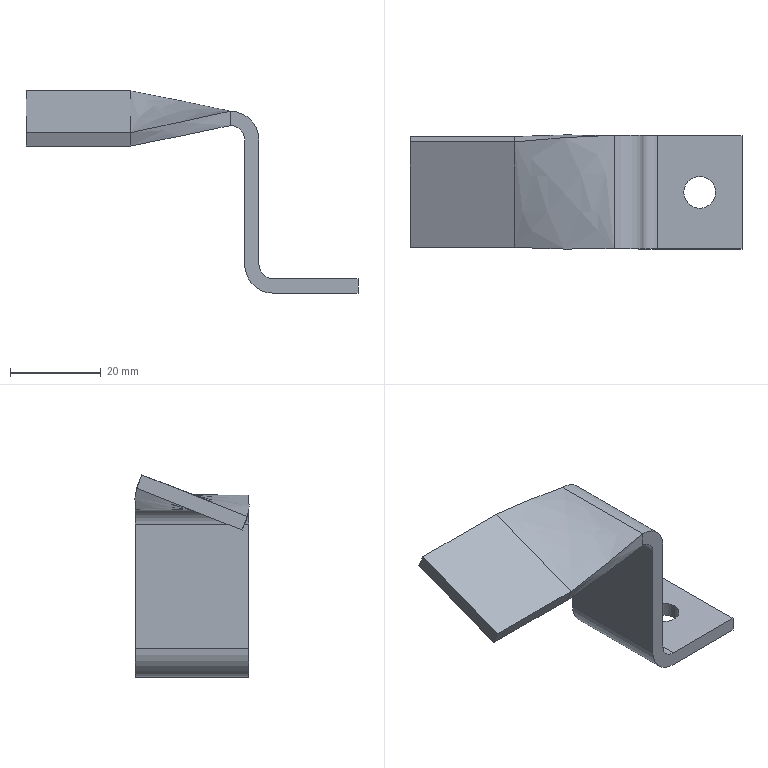Part | SolidWorks | features BaseBody 1 | 1 solid | 24 faces | box 73.18 x 25.199 x 44.598 mm | volume 8281 mm3 | plane 14 | cylinder 6 | spline 4 | commonest cylinder face diameters 6.34 x2 7 x2 12.68 x2
STEP:
#1=CARTESIAN_POINT('',(1.209,1.044,3.17));
#2=VERTEX_POINT('',#1);
#3=CARTESIAN_POINT('',(-5.791,1.044,3.17));
#4=VERTEX_POINT('',#3);
#5=CARTESIAN_POINT('',(-2.291,1.044,3.17));
#6=DIRECTION('',(0.,0.,-1.));
#7=DIRECTION('',(-1.,0.,0.));
#8=AXIS2_PLACEMENT_3D('',#5,#6,#7);
#9=CIRCLE('',#8,3.5);
#10=EDGE_CURVE('',#2,#4,#9,.T.);
#11=ORIENTED_EDGE('',*,*,#10,.F.);
#12=CARTESIAN_POINT('',(1.209,1.044,0.));
#13=VERTEX_POINT('',#12);
#14=CARTESIAN_POINT('',(1.209,1.044,89.394));
#15=DIRECTION('',(0.,0.,-1.));
#16=VECTOR('',#15,1000.);
#17=LINE('',#14,#16);
#18=EDGE_CURVE('',#2,#13,#17,.T.);
#19=ORIENTED_EDGE('',*,*,#18,.T.);
#20=CARTESIAN_POINT('',(-5.791,1.044,0.));
#21=VERTEX_POINT('',#20);
#22=CARTESIAN_POINT('',(-2.291,1.044,0.));
#23=DIRECTION('',(0.,0.,-1.));
#24=DIRECTION('',(-1.,0.,0.));
#25=AXIS2_PLACEMENT_3D('',#22,#23,#24);
#26=CIRCLE('',#25,3.5);
#27=EDGE_CURVE('',#13,#21,#26,.T.);
#28=ORIENTED_EDGE('',*,*,#27,.T.);
#29=CARTESIAN_POINT('',(-5.791,1.044,89.394));
#30=DIRECTION('',(0.,0.,-1.));
#31=VECTOR('',#30,1000.);
#32=LINE('',#29,#31);
#33=EDGE_CURVE('',#4,#21,#32,.T.);
#34=ORIENTED_EDGE('',*,*,#33,.F.);
#35=EDGE_LOOP('',(#11,#19,#28,#34));
#36=FACE_OUTER_BOUND('',#35,.T.);
#37=CARTESIAN_POINT('',(-2.291,1.044,89.394));
#38=DIRECTION('',(0.,0.,-1.));
#39=DIRECTION('',(-1.,0.,0.));
#40=AXIS2_PLACEMENT_3D('',#37,#38,#39);
#41=CYLINDRICAL_SURFACE('',#40,3.5);
#42=ADVANCED_FACE('',(#36),#41,.F.);
#43=CARTESIAN_POINT('',(-14.791,-11.456,6.34));
#44=VERTEX_POINT('',#43);
#45=CARTESIAN_POINT('',(-14.791,13.544,6.34));
#46=VERTEX_POINT('',#45);
#47=CARTESIAN_POINT('',(-14.791,13.544,6.34));
#48=DIRECTION('',(0.,1.,0.));
#49=VECTOR('',#48,1000.);
#50=LINE('',#47,#49);
#51=EDGE_CURVE('',#44,#46,#50,.T.);
#52=ORIENTED_EDGE('',*,*,#51,.T.);
#53=CARTESIAN_POINT('',(-14.791,13.544,33.76));
#54=VERTEX_POINT('',#53);
#55=CARTESIAN_POINT('',(-14.791,13.544,40.1));
#56=DIRECTION('',(0.,0.,1.));
#57=VECTOR('',#56,1000.);
#58=LINE('',#55,#57);
#59=EDGE_CURVE('',#46,#54,#58,.T.);
#60=ORIENTED_EDGE('',*,*,#59,.T.);
#61=CARTESIAN_POINT('',(-14.791,-11.456,33.76));
#62=VERTEX_POINT('',#61);
#63=CARTESIAN_POINT('',(-14.791,13.544,33.76));
#64=DIRECTION('',(0.,-1.,0.));
#65=VECTOR('',#64,1000.);
#66=LINE('',#63,#65);
#67=EDGE_CURVE('',#54,#62,#66,.T.);
#68=ORIENTED_EDGE('',*,*,#67,.T.);
#69=CARTESIAN_POINT('',(-14.791,-11.456,40.1));
#70=DIRECTION('',(0.,0.,-1.));
#71=VECTOR('',#70,1000.);
#72=LINE('',#69,#71);
#73=EDGE_CURVE('',#62,#44,#72,.T.);
#74=ORIENTED_EDGE('',*,*,#73,.T.);
#75=EDGE_LOOP('',(#52,#60,#68,#74));
#76=FACE_OUTER_BOUND('',#75,.T.);
#77=CARTESIAN_POINT('',(-14.791,13.544,40.1));
#78=DIRECTION('',(1.,0.,0.));
#79=DIRECTION('',(0.,1.,0.));
#80=AXIS2_PLACEMENT_3D('',#77,#78,#79);
#81=PLANE('',#80);
#82=ADVANCED_FACE('',(#76),#81,.T.);
#83=CARTESIAN_POINT('',(-17.961,13.544,6.34));
#84=VERTEX_POINT('',#83);
#85=CARTESIAN_POINT('',(-17.961,13.544,33.76));
#86=VERTEX_POINT('',#85);
#87=CARTESIAN_POINT('',(-17.961,13.544,38.515));
#88=DIRECTION('',(0.,0.,1.));
#89=VECTOR('',#88,1000.);
#90=LINE('',#87,#89);
#91=EDGE_CURVE('',#84,#86,#90,.T.);
#92=ORIENTED_EDGE('',*,*,#91,.T.);
#93=CARTESIAN_POINT('',(-21.131,13.544,36.93));
#94=VERTEX_POINT('',#93);
#95=CARTESIAN_POINT('',(-21.131,13.544,33.76));
#96=DIRECTION('',(0.,-1.,0.));
#97=DIRECTION('',(1.,0.,0.));
#98=AXIS2_PLACEMENT_3D('',#95,#96,#97);
#99=CIRCLE('',#98,3.17);
#100=EDGE_CURVE('',#86,#94,#99,.T.);
#101=ORIENTED_EDGE('',*,*,#100,.T.);
#102=CARTESIAN_POINT('',(-21.141,13.544,36.93));
#103=VERTEX_POINT('',#102);
#104=CARTESIAN_POINT('',(-21.141,13.544,36.93));
#105=DIRECTION('',(1.,0.,0.));
#106=VECTOR('',#105,1000.);
#107=LINE('',#104,#106);
#108=EDGE_CURVE('',#103,#94,#107,.T.);
#109=ORIENTED_EDGE('',*,*,#108,.F.);
#110=CARTESIAN_POINT('',(-21.141,13.544,40.1));
#111=VERTEX_POINT('',#110);
#112=CARTESIAN_POINT('',(-21.141,13.544,38.515));
#113=DIRECTION('',(0.,0.,-1.));
#114=VECTOR('',#113,1000.);
#115=LINE('',#112,#114);
#116=EDGE_CURVE('',#111,#103,#115,.T.);
#117=ORIENTED_EDGE('',*,*,#116,.F.);
#118=CARTESIAN_POINT('',(-21.131,13.544,40.1));
#119=VERTEX_POINT('',#118);
#120=CARTESIAN_POINT('',(-14.791,13.544,40.1));
#121=DIRECTION('',(-1.,0.,0.));
#122=VECTOR('',#121,1000.);
#123=LINE('',#120,#122);
#124=EDGE_CURVE('',#119,#111,#123,.T.);
#125=ORIENTED_EDGE('',*,*,#124,.F.);
#126=CARTESIAN_POINT('',(-21.131,13.544,33.76));
#127=DIRECTION('',(0.,1.,0.));
#128=DIRECTION('',(1.,0.,0.));
#129=AXIS2_PLACEMENT_3D('',#126,#127,#128);
#130=CIRCLE('',#129,6.34);
#131=EDGE_CURVE('',#119,#54,#130,.T.);
#132=ORIENTED_EDGE('',*,*,#131,.T.);
#133=ORIENTED_EDGE('',*,*,#59,.F.);
#134=CARTESIAN_POINT('',(-11.621,13.544,3.17));
#135=VERTEX_POINT('',#134);
#136=CARTESIAN_POINT('',(-11.621,13.544,6.34));
#137=DIRECTION('',(0.,-1.,0.));
#138=DIRECTION('',(-1.,0.,0.));
#139=AXIS2_PLACEMENT_3D('',#136,#137,#138);
#140=CIRCLE('',#139,3.17);
#141=EDGE_CURVE('',#46,#135,#140,.T.);
#142=ORIENTED_EDGE('',*,*,#141,.T.);
#143=CARTESIAN_POINT('',(7.039,13.544,3.17));
#144=VERTEX_POINT('',#143);
#145=CARTESIAN_POINT('',(-17.966,13.544,3.17));
#146=DIRECTION('',(1.,0.,0.));
#147=VECTOR('',#146,1000.);
#148=LINE('',#145,#147);
#149=EDGE_CURVE('',#135,#144,#148,.T.);
#150=ORIENTED_EDGE('',*,*,#149,.T.);
#151=CARTESIAN_POINT('',(7.039,13.544,0.));
#152=VERTEX_POINT('',#151);
#153=CARTESIAN_POINT('',(7.039,13.544,38.515));
#154=DIRECTION('',(0.,0.,-1.));
#155=VECTOR('',#154,1000.);
#156=LINE('',#153,#155);
#157=EDGE_CURVE('',#144,#152,#156,.T.);
#158=ORIENTED_EDGE('',*,*,#157,.T.);
#159=CARTESIAN_POINT('',(-11.621,13.544,0.));
#160=VERTEX_POINT('',#159);
#161=CARTESIAN_POINT('',(-17.966,13.544,0.));
#162=DIRECTION('',(-1.,0.,0.));
#163=VECTOR('',#162,1000.);
#164=LINE('',#161,#163);
#165=EDGE_CURVE('',#152,#160,#164,.T.);
#166=ORIENTED_EDGE('',*,*,#165,.T.);
#167=CARTESIAN_POINT('',(-11.621,13.544,6.34));
#168=DIRECTION('',(0.,1.,0.));
#169=DIRECTION('',(-1.,0.,0.));
#170=AXIS2_PLACEMENT_3D('',#167,#168,#169);
#171=CIRCLE('',#170,6.34);
#172=EDGE_CURVE('',#160,#84,#171,.T.);
#173=ORIENTED_EDGE('',*,*,#172,.T.);
#174=EDGE_LOOP('',(#92,#101,#109,#117,#125,#132,#133,#142,#150,#158,#166,#173));
#175=FACE_OUTER_BOUND('',#174,.T.);
#176=CARTESIAN_POINT('',(-17.966,13.544,38.515));
#177=DIRECTION('',(0.,1.,0.));
#178=DIRECTION('',(0.,0.,1.));
#179=AXIS2_PLACEMENT_3D('',#176,#177,#178);
#180=PLANE('',#179);
#181=ADVANCED_FACE('',(#175),#180,.T.);
#182=CARTESIAN_POINT('',(-11.621,-11.456,3.17));
#183=VERTEX_POINT('',#182);
#184=CARTESIAN_POINT('',(-11.621,-11.456,6.34));
#185=DIRECTION('',(0.,1.,0.));
#186=DIRECTION('',(-1.,0.,0.));
#187=AXIS2_PLACEMENT_3D('',#184,#185,#186);
#188=CIRCLE('',#187,3.17);
#189=EDGE_CURVE('',#183,#44,#188,.T.);
#190=ORIENTED_EDGE('',*,*,#189,.F.);
#191=CARTESIAN_POINT('',(-11.621,1.044,3.17));
#192=DIRECTION('',(0.,-1.,0.));
#193=VECTOR('',#192,1000.);
#194=LINE('',#191,#193);
#195=EDGE_CURVE('',#135,#183,#194,.T.);
#196=ORIENTED_EDGE('',*,*,#195,.F.);
#197=ORIENTED_EDGE('',*,*,#141,.F.);
#198=ORIENTED_EDGE('',*,*,#51,.F.);
#199=EDGE_LOOP('',(#190,#196,#197,#198));
#200=FACE_OUTER_BOUND('',#199,.T.);
#201=CARTESIAN_POINT('',(-11.621,1.044,6.34));
#202=DIRECTION('',(0.,1.,0.));
#203=DIRECTION('',(-1.,0.,0.));
#204=AXIS2_PLACEMENT_3D('',#201,#202,#203);
#205=CYLINDRICAL_SURFACE('',#204,3.17);
#206=ADVANCED_FACE('',(#200),#205,.F.);
#207=CARTESIAN_POINT('',(-21.141,-11.456,36.93));
#208=VERTEX_POINT('',#207);
#209=CARTESIAN_POINT('',(-21.141,-11.456,40.1));
#210=VERTEX_POINT('',#209);
#211=CARTESIAN_POINT('',(-21.141,-11.456,38.515));
#212=DIRECTION('',(0.,0.,1.));
#213=VECTOR('',#212,1000.);
#214=LINE('',#211,#213);
#215=EDGE_CURVE('',#208,#210,#214,.T.);
#216=ORIENTED_EDGE('',*,*,#215,.F.);
#217=CARTESIAN_POINT('',(-21.131,-11.456,36.93));
#218=VERTEX_POINT('',#217);
#219=CARTESIAN_POINT('',(-21.141,-11.456,36.93));
#220=DIRECTION('',(-1.,0.,0.));
#221=VECTOR('',#220,1000.);
#222=LINE('',#219,#221);
#223=EDGE_CURVE('',#218,#208,#222,.T.);
#224=ORIENTED_EDGE('',*,*,#223,.F.);
#225=CARTESIAN_POINT('',(-17.961,-11.456,33.76));
#226=VERTEX_POINT('',#225);
#227=CARTESIAN_POINT('',(-21.131,-11.456,33.76));
#228=DIRECTION('',(0.,-1.,0.));
#229=DIRECTION('',(1.,0.,0.));
#230=AXIS2_PLACEMENT_3D('',#227,#228,#229);
#231=CIRCLE('',#230,3.17);
#232=EDGE_CURVE('',#226,#218,#231,.T.);
#233=ORIENTED_EDGE('',*,*,#232,.F.);
#234=CARTESIAN_POINT('',(-17.961,-11.456,6.34));
#235=VERTEX_POINT('',#234);
#236=CARTESIAN_POINT('',(-17.961,-11.456,38.515));
#237=DIRECTION('',(0.,0.,1.));
#238=VECTOR('',#237,1000.);
#239=LINE('',#236,#238);
#240=EDGE_CURVE('',#235,#226,#239,.T.);
#241=ORIENTED_EDGE('',*,*,#240,.F.);
#242=CARTESIAN_POINT('',(-11.621,-11.456,0.));
#243=VERTEX_POINT('',#242);
#244=CARTESIAN_POINT('',(-11.621,-11.456,6.34));
#245=DIRECTION('',(0.,1.,0.));
#246=DIRECTION('',(-1.,0.,0.));
#247=AXIS2_PLACEMENT_3D('',#244,#245,#246);
#248=CIRCLE('',#247,6.34);
#249=EDGE_CURVE('',#243,#235,#248,.T.);
#250=ORIENTED_EDGE('',*,*,#249,.F.);
#251=CARTESIAN_POINT('',(7.039,-11.456,0.));
#252=VERTEX_POINT('',#251);
#253=CARTESIAN_POINT('',(-17.966,-11.456,0.));
#254=DIRECTION('',(-1.,0.,0.));
#255=VECTOR('',#254,1000.);
#256=LINE('',#253,#255);
#257=EDGE_CURVE('',#252,#243,#256,.T.);
#258=ORIENTED_EDGE('',*,*,#257,.F.);
#259=CARTESIAN_POINT('',(7.039,-11.456,3.17));
#260=VERTEX_POINT('',#259);
#261=CARTESIAN_POINT('',(7.039,-11.456,38.515));
#262=DIRECTION('',(0.,0.,-1.));
#263=VECTOR('',#262,1000.);
#264=LINE('',#261,#263);
#265=EDGE_CURVE('',#260,#252,#264,.T.);
#266=ORIENTED_EDGE('',*,*,#265,.F.);
#267=CARTESIAN_POINT('',(-17.966,-11.456,3.17));
#268=DIRECTION('',(1.,0.,0.));
#269=VECTOR('',#268,1000.);
#270=LINE('',#267,#269);
#271=EDGE_CURVE('',#183,#260,#270,.T.);
#272=ORIENTED_EDGE('',*,*,#271,.F.);
#273=ORIENTED_EDGE('',*,*,#189,.T.);
#274=ORIENTED_EDGE('',*,*,#73,.F.);
#275=CARTESIAN_POINT('',(-21.131,-11.456,40.1));
#276=VERTEX_POINT('',#275);
#277=CARTESIAN_POINT('',(-21.131,-11.456,33.76));
#278=DIRECTION('',(0.,1.,0.));
#279=DIRECTION('',(1.,0.,0.));
#280=AXIS2_PLACEMENT_3D('',#277,#278,#279);
#281=CIRCLE('',#280,6.34);
#282=EDGE_CURVE('',#276,#62,#281,.T.);
#283=ORIENTED_EDGE('',*,*,#282,.F.);
#284=CARTESIAN_POINT('',(-14.791,-11.456,40.1));
#285=DIRECTION('',(1.,0.,0.));
#286=VECTOR('',#285,1000.);
#287=LINE('',#284,#286);
#288=EDGE_CURVE('',#210,#276,#287,.T.);
#289=ORIENTED_EDGE('',*,*,#288,.F.);
#290=EDGE_LOOP('',(#216,#224,#233,#241,#250,#258,#266,#272,#273,#274,#283,#289));
#291=FACE_OUTER_BOUND('',#290,.T.);
#292=CARTESIAN_POINT('',(-17.966,-11.456,38.515));
#293=DIRECTION('',(0.,1.,0.));
#294=DIRECTION('',(0.,0.,1.));
#295=AXIS2_PLACEMENT_3D('',#292,#293,#294);
#296=PLANE('',#295);
#297=ADVANCED_FACE('',(#291),#296,.F.);
#298=ORIENTED_EDGE('',*,*,#67,.F.);
#299=ORIENTED_EDGE('',*,*,#131,.F.);
#300=CARTESIAN_POINT('',(-21.131,1.044,40.1));
#301=DIRECTION('',(0.,-1.,0.));
#302=VECTOR('',#301,1000.);
#303=LINE('',#300,#302);
#304=EDGE_CURVE('',#119,#276,#303,.T.);
#305=ORIENTED_EDGE('',*,*,#304,.T.);
#306=ORIENTED_EDGE('',*,*,#282,.T.);
#307=EDGE_LOOP('',(#298,#299,#305,#306));
#308=FACE_OUTER_BOUND('',#307,.T.);
#309=CARTESIAN_POINT('',(-21.131,1.044,33.76));
#310=DIRECTION('',(0.,-1.,0.));
#311=DIRECTION('',(1.,0.,0.));
#312=AXIS2_PLACEMENT_3D('',#309,#310,#311);
#313=CYLINDRICAL_SURFACE('',#312,6.34);
#314=ADVANCED_FACE('',(#308),#313,.T.);
#315=ORIENTED_EDGE('',*,*,#100,.F.);
#316=CARTESIAN_POINT('',(-17.961,1.044,33.76));
#317=DIRECTION('',(0.,1.,0.));
#318=VECTOR('',#317,1000.);
#319=LINE('',#316,#318);
#320=EDGE_CURVE('',#226,#86,#319,.T.);
#321=ORIENTED_EDGE('',*,*,#320,.F.);
#322=ORIENTED_EDGE('',*,*,#232,.T.);
#323=CARTESIAN_POINT('',(-21.131,1.044,36.93));
#324=DIRECTION('',(0.,-1.,0.));
#325=VECTOR('',#324,1000.);
#326=LINE('',#323,#325);
#327=EDGE_CURVE('',#94,#218,#326,.T.);
#328=ORIENTED_EDGE('',*,*,#327,.F.);
#329=EDGE_LOOP('',(#315,#321,#322,#328));
#330=FACE_OUTER_BOUND('',#329,.T.);
#331=CARTESIAN_POINT('',(-21.131,1.044,33.76));
#332=DIRECTION('',(0.,-1.,0.));
#333=DIRECTION('',(1.,0.,0.));
#334=AXIS2_PLACEMENT_3D('',#331,#332,#333);
#335=CYLINDRICAL_SURFACE('',#334,3.17);
#336=ADVANCED_FACE('',(#330),#335,.F.);
#337=CARTESIAN_POINT('',(-17.961,13.544,6.34));
#338=DIRECTION('',(0.,-1.,0.));
#339=VECTOR('',#338,1000.);
#340=LINE('',#337,#339);
#341=EDGE_CURVE('',#84,#235,#340,.T.);
#342=ORIENTED_EDGE('',*,*,#341,.T.);
#343=ORIENTED_EDGE('',*,*,#240,.T.);
#344=ORIENTED_EDGE('',*,*,#320,.T.);
#345=ORIENTED_EDGE('',*,*,#91,.F.);
#346=EDGE_LOOP('',(#342,#343,#344,#345));
#347=FACE_OUTER_BOUND('',#346,.T.);
#348=CARTESIAN_POINT('',(-17.961,13.544,0.));
#349=DIRECTION('',(-1.,0.,0.));
#350=DIRECTION('',(0.,-1.,0.));
#351=AXIS2_PLACEMENT_3D('',#348,#349,#350);
#352=PLANE('',#351);
#353=ADVANCED_FACE('',(#347),#352,.T.);
#354=CARTESIAN_POINT('',(-11.621,1.044,0.));
#355=DIRECTION('',(0.,-1.,0.));
#356=VECTOR('',#355,1000.);
#357=LINE('',#354,#356);
#358=EDGE_CURVE('',#160,#243,#357,.T.);
#359=ORIENTED_EDGE('',*,*,#358,.T.);
#360=ORIENTED_EDGE('',*,*,#249,.T.);
#361=ORIENTED_EDGE('',*,*,#341,.F.);
#362=ORIENTED_EDGE('',*,*,#172,.F.);
#363=EDGE_LOOP('',(#359,#360,#361,#362));
#364=FACE_OUTER_BOUND('',#363,.T.);
#365=CARTESIAN_POINT('',(-11.621,1.044,6.34));
#366=DIRECTION('',(0.,1.,0.));
#367=DIRECTION('',(-1.,0.,0.));
#368=AXIS2_PLACEMENT_3D('',#365,#366,#367);
#369=CYLINDRICAL_SURFACE('',#368,6.34);
#370=ADVANCED_FACE('',(#364),#369,.T.);
#371=CARTESIAN_POINT('',(-2.291,1.044,0.));
#372=DIRECTION('',(0.,0.,-1.));
#373=DIRECTION('',(-1.,0.,0.));
#374=AXIS2_PLACEMENT_3D('',#371,#372,#373);
#375=CIRCLE('',#374,3.5);
#376=EDGE_CURVE('',#21,#13,#375,.T.);
#377=ORIENTED_EDGE('',*,*,#376,.F.);
#378=ORIENTED_EDGE('',*,*,#27,.F.);
#379=EDGE_LOOP('',(#377,#378));
#380=FACE_BOUND('',#379,.T.);
#381=ORIENTED_EDGE('',*,*,#165,.F.);
#382=CARTESIAN_POINT('',(7.039,1.044,0.));
#383=DIRECTION('',(0.,1.,0.));
#384=VECTOR('',#383,1000.);
#385=LINE('',#382,#384);
#386=EDGE_CURVE('',#252,#152,#385,.T.);
#387=ORIENTED_EDGE('',*,*,#386,.F.);
#388=ORIENTED_EDGE('',*,*,#257,.T.);
#389=ORIENTED_EDGE('',*,*,#358,.F.);
#390=EDGE_LOOP('',(#381,#387,#388,#389));
#391=FACE_OUTER_BOUND('',#390,.T.);
#392=CARTESIAN_POINT('',(-5.461,1.044,0.));
#393=DIRECTION('',(0.,0.,1.));
#394=DIRECTION('',(1.,0.,0.));
#395=AXIS2_PLACEMENT_3D('',#392,#393,#394);
#396=PLANE('',#395);
#397=ADVANCED_FACE('',(#380,#391),#396,.F.);
#398=ORIENTED_EDGE('',*,*,#386,.T.);
#399=ORIENTED_EDGE('',*,*,#157,.F.);
#400=CARTESIAN_POINT('',(7.039,13.544,3.17));
#401=DIRECTION('',(0.,-1.,0.));
#402=VECTOR('',#401,1000.);
#403=LINE('',#400,#402);
#404=EDGE_CURVE('',#144,#260,#403,.T.);
#405=ORIENTED_EDGE('',*,*,#404,.T.);
#406=ORIENTED_EDGE('',*,*,#265,.T.);
#407=EDGE_LOOP('',(#398,#399,#405,#406));
#408=FACE_OUTER_BOUND('',#407,.T.);
#409=CARTESIAN_POINT('',(7.039,13.544,0.));
#410=DIRECTION('',(1.,0.,0.));
#411=DIRECTION('',(0.,0.,-1.));
#412=AXIS2_PLACEMENT_3D('',#409,#410,#411);
#413=PLANE('',#412);
#414=ADVANCED_FACE('',(#408),#413,.T.);
#415=CARTESIAN_POINT('',(-2.291,1.044,3.17));
#416=DIRECTION('',(0.,0.,-1.));
#417=DIRECTION('',(-1.,0.,0.));
#418=AXIS2_PLACEMENT_3D('',#415,#416,#417);
#419=CIRCLE('',#418,3.5);
#420=EDGE_CURVE('',#4,#2,#419,.T.);
#421=ORIENTED_EDGE('',*,*,#420,.T.);
#422=ORIENTED_EDGE('',*,*,#10,.T.);
#423=EDGE_LOOP('',(#421,#422));
#424=FACE_BOUND('',#423,.T.);
#425=ORIENTED_EDGE('',*,*,#404,.F.);
#426=ORIENTED_EDGE('',*,*,#149,.F.);
#427=ORIENTED_EDGE('',*,*,#195,.T.);
#428=ORIENTED_EDGE('',*,*,#271,.T.);
#429=EDGE_LOOP('',(#425,#426,#427,#428));
#430=FACE_OUTER_BOUND('',#429,.T.);
#431=CARTESIAN_POINT('',(-5.461,1.044,3.17));
#432=DIRECTION('',(0.,0.,1.));
#433=DIRECTION('',(1.,0.,0.));
#434=AXIS2_PLACEMENT_3D('',#431,#432,#433);
#435=PLANE('',#434);
#436=ADVANCED_FACE('',(#424,#430),#435,.T.);
#437=CARTESIAN_POINT('',(-21.141,-11.456,40.1));
#438=DIRECTION('',(0.,-1.,0.));
#439=VECTOR('',#438,1000.);
#440=LINE('',#437,#439);
#441=EDGE_CURVE('',#111,#210,#440,.T.);
#442=ORIENTED_EDGE('',*,*,#441,.T.);
#443=ORIENTED_EDGE('',*,*,#288,.T.);
#444=ORIENTED_EDGE('',*,*,#304,.F.);
#445=ORIENTED_EDGE('',*,*,#124,.T.);
#446=EDGE_LOOP('',(#442,#443,#444,#445));
#447=FACE_OUTER_BOUND('',#446,.T.);
#448=CARTESIAN_POINT('',(-14.791,-11.456,40.1));
#449=DIRECTION('',(0.,0.,1.));
#450=DIRECTION('',(1.,0.,0.));
#451=AXIS2_PLACEMENT_3D('',#448,#449,#450);
#452=PLANE('',#451);
#453=ADVANCED_FACE('',(#447),#452,.T.);
#454=CARTESIAN_POINT('',(-21.141,-11.456,36.93));
#455=DIRECTION('',(0.,1.,0.));
#456=VECTOR('',#455,1000.);
#457=LINE('',#454,#456);
#458=EDGE_CURVE('',#208,#103,#457,.T.);
#459=ORIENTED_EDGE('',*,*,#458,.T.);
#460=ORIENTED_EDGE('',*,*,#108,.T.);
#461=ORIENTED_EDGE('',*,*,#327,.T.);
#462=ORIENTED_EDGE('',*,*,#223,.T.);
#463=EDGE_LOOP('',(#459,#460,#461,#462));
#464=FACE_OUTER_BOUND('',#463,.T.);
#465=CARTESIAN_POINT('',(-21.141,-11.456,36.93));
#466=DIRECTION('',(0.,0.,-1.));
#467=DIRECTION('',(-1.,0.,0.));
#468=AXIS2_PLACEMENT_3D('',#465,#466,#467);
#469=PLANE('',#468);
#470=ADVANCED_FACE('',(#464),#469,.T.);
#471=ORIENTED_EDGE('',*,*,#18,.F.);
#472=ORIENTED_EDGE('',*,*,#420,.F.);
#473=ORIENTED_EDGE('',*,*,#33,.T.);
#474=ORIENTED_EDGE('',*,*,#376,.T.);
#475=EDGE_LOOP('',(#471,#472,#473,#474));
#476=FACE_OUTER_BOUND('',#475,.T.);
#477=CARTESIAN_POINT('',(-2.291,1.044,89.394));
#478=DIRECTION('',(0.,0.,-1.));
#479=DIRECTION('',(-1.,0.,0.));
#480=AXIS2_PLACEMENT_3D('',#477,#478,#479);
#481=CYLINDRICAL_SURFACE('',#480,3.5);
#482=ADVANCED_FACE('',(#476),#481,.F.);
#483=ORIENTED_EDGE('',*,*,#441,.F.);
#484=CARTESIAN_POINT('',(-43.141,12.078,44.598));
#485=VERTEX_POINT('',#484);
#486=CARTESIAN_POINT('',(-21.141,13.544,40.1));
#487=CARTESIAN_POINT('',(-28.474,13.344,41.674));
#488=CARTESIAN_POINT('',(-35.808,12.844,43.209));
#489=CARTESIAN_POINT('',(-43.141,12.078,44.598));
#490=B_SPLINE_CURVE_WITH_KNOTS('',3,(#486,#487,#488,#489),.UNSPECIFIED.,.F.,.F.,(4,4),(0.,0.3777),.UNSPECIFIED.);
#491=EDGE_CURVE('',#111,#485,#490,.T.);
#492=ORIENTED_EDGE('',*,*,#491,.T.);
#493=CARTESIAN_POINT('',(-43.141,-11.16,35.379));
#494=VERTEX_POINT('',#493);
#495=CARTESIAN_POINT('',(-43.141,0.4592,39.988));
#496=DIRECTION('',(0.,-0.9295,-0.3688));
#497=VECTOR('',#496,1000.);
#498=LINE('',#495,#497);
#499=EDGE_CURVE('',#485,#494,#498,.T.);
#500=ORIENTED_EDGE('',*,*,#499,.T.);
#501=CARTESIAN_POINT('',(-43.141,-11.16,35.379));
#502=CARTESIAN_POINT('',(-35.808,-11.555,36.915));
#503=CARTESIAN_POINT('',(-28.474,-11.656,38.526));
#504=CARTESIAN_POINT('',(-21.141,-11.456,40.1));
#505=B_SPLINE_CURVE_WITH_KNOTS('',3,(#501,#502,#503,#504),.UNSPECIFIED.,.F.,.F.,(4,4),(0.,0.3777),.UNSPECIFIED.);
#506=EDGE_CURVE('',#494,#210,#505,.T.);
#507=ORIENTED_EDGE('',*,*,#506,.T.);
#508=EDGE_LOOP('',(#483,#492,#500,#507));
#509=FACE_OUTER_BOUND('',#508,.T.);
#510=CARTESIAN_POINT('',(-21.141,-11.456,40.1));
#511=CARTESIAN_POINT('',(-28.474,-11.656,38.526));
#512=CARTESIAN_POINT('',(-35.808,-11.555,36.915));
#513=CARTESIAN_POINT('',(-43.141,-11.16,35.379));
#514=CARTESIAN_POINT('',(-21.141,-3.123,40.1));
#515=CARTESIAN_POINT('',(-28.474,-3.323,39.575));
#516=CARTESIAN_POINT('',(-35.808,-3.422,39.013));
#517=CARTESIAN_POINT('',(-43.141,-3.414,38.452));
#518=CARTESIAN_POINT('',(-21.141,5.21,40.1));
#519=CARTESIAN_POINT('',(-28.474,5.011,40.625));
#520=CARTESIAN_POINT('',(-35.808,4.711,41.111));
#521=CARTESIAN_POINT('',(-43.141,4.332,41.525));
#522=CARTESIAN_POINT('',(-21.141,13.544,40.1));
#523=CARTESIAN_POINT('',(-28.474,13.344,41.674));
#524=CARTESIAN_POINT('',(-35.808,12.844,43.209));
#525=CARTESIAN_POINT('',(-43.141,12.078,44.598));
#526=B_SPLINE_SURFACE_WITH_KNOTS('',3,3,((#510,#511,#512,#513),(#514,#515,#516,#517),(#518,#519,#520,#521),(#522,#523,#524,#525)),.UNSPECIFIED.,.F.,.F.,.F.,(4,4),(4,4),(0.,2.5),(0.,0.3777),.UNSPECIFIED.);
#527=ADVANCED_FACE('',(#509),#526,.T.);
#528=ORIENTED_EDGE('',*,*,#458,.F.);
#529=CARTESIAN_POINT('',(-43.141,-9.991,32.432));
#530=VERTEX_POINT('',#529);
#531=CARTESIAN_POINT('',(-21.141,-11.456,36.93));
#532=CARTESIAN_POINT('',(-28.474,-11.257,35.356));
#533=CARTESIAN_POINT('',(-35.808,-10.757,33.821));
#534=CARTESIAN_POINT('',(-43.141,-9.991,32.432));
#535=B_SPLINE_CURVE_WITH_KNOTS('',3,(#531,#532,#533,#534),.UNSPECIFIED.,.F.,.F.,(4,4),(0.,0.3777),.UNSPECIFIED.);
#536=EDGE_CURVE('',#208,#530,#535,.T.);
#537=ORIENTED_EDGE('',*,*,#536,.T.);
#538=CARTESIAN_POINT('',(-43.141,13.247,41.651));
#539=VERTEX_POINT('',#538);
#540=CARTESIAN_POINT('',(-43.141,1.628,37.042));
#541=DIRECTION('',(0.,0.9295,0.3688));
#542=VECTOR('',#541,1000.);
#543=LINE('',#540,#542);
#544=EDGE_CURVE('',#530,#539,#543,.T.);
#545=ORIENTED_EDGE('',*,*,#544,.T.);
#546=CARTESIAN_POINT('',(-43.141,13.247,41.651));
#547=CARTESIAN_POINT('',(-35.808,13.642,40.115));
#548=CARTESIAN_POINT('',(-28.474,13.743,38.504));
#549=CARTESIAN_POINT('',(-21.141,13.544,36.93));
#550=B_SPLINE_CURVE_WITH_KNOTS('',3,(#546,#547,#548,#549),.UNSPECIFIED.,.F.,.F.,(4,4),(0.,0.3777),.UNSPECIFIED.);
#551=EDGE_CURVE('',#539,#103,#550,.T.);
#552=ORIENTED_EDGE('',*,*,#551,.T.);
#553=EDGE_LOOP('',(#528,#537,#545,#552));
#554=FACE_OUTER_BOUND('',#553,.T.);
#555=CARTESIAN_POINT('',(-21.141,13.544,36.93));
#556=CARTESIAN_POINT('',(-28.474,13.743,38.504));
#557=CARTESIAN_POINT('',(-35.808,13.642,40.115));
#558=CARTESIAN_POINT('',(-43.141,13.247,41.651));
#559=CARTESIAN_POINT('',(-21.141,5.21,36.93));
#560=CARTESIAN_POINT('',(-28.474,5.41,37.455));
#561=CARTESIAN_POINT('',(-35.808,5.509,38.017));
#562=CARTESIAN_POINT('',(-43.141,5.501,38.578));
#563=CARTESIAN_POINT('',(-21.141,-3.123,36.93));
#564=CARTESIAN_POINT('',(-28.474,-2.923,36.405));
#565=CARTESIAN_POINT('',(-35.808,-2.624,35.919));
#566=CARTESIAN_POINT('',(-43.141,-2.245,35.505));
#567=CARTESIAN_POINT('',(-21.141,-11.456,36.93));
#568=CARTESIAN_POINT('',(-28.474,-11.257,35.356));
#569=CARTESIAN_POINT('',(-35.808,-10.757,33.821));
#570=CARTESIAN_POINT('',(-43.141,-9.991,32.432));
#571=B_SPLINE_SURFACE_WITH_KNOTS('',3,3,((#555,#556,#557,#558),(#559,#560,#561,#562),(#563,#564,#565,#566),(#567,#568,#569,#570)),.UNSPECIFIED.,.F.,.F.,.F.,(4,4),(4,4),(0.,2.5),(0.,0.3777),.UNSPECIFIED.);
#572=ADVANCED_FACE('',(#554),#571,.T.);
#573=ORIENTED_EDGE('',*,*,#116,.T.);
#574=ORIENTED_EDGE('',*,*,#551,.F.);
#575=CARTESIAN_POINT('',(-43.141,13.247,41.651));
#576=DIRECTION('',(0.,0.3688,-0.9295));
#577=VECTOR('',#576,1000.);
#578=LINE('',#575,#577);
#579=EDGE_CURVE('',#485,#539,#578,.T.);
#580=ORIENTED_EDGE('',*,*,#579,.F.);
#581=ORIENTED_EDGE('',*,*,#491,.F.);
#582=EDGE_LOOP('',(#573,#574,#580,#581));
#583=FACE_OUTER_BOUND('',#582,.T.);
#584=CARTESIAN_POINT('',(-21.141,13.544,40.1));
#585=CARTESIAN_POINT('',(-28.474,13.344,41.674));
#586=CARTESIAN_POINT('',(-35.808,12.844,43.209));
#587=CARTESIAN_POINT('',(-43.141,12.078,44.598));
#588=CARTESIAN_POINT('',(-21.141,13.544,39.043));
#589=CARTESIAN_POINT('',(-28.474,13.477,40.617));
#590=CARTESIAN_POINT('',(-35.808,13.11,42.177));
#591=CARTESIAN_POINT('',(-43.141,12.468,43.616));
#592=CARTESIAN_POINT('',(-21.141,13.544,37.987));
#593=CARTESIAN_POINT('',(-28.474,13.61,39.56));
#594=CARTESIAN_POINT('',(-35.808,13.376,41.146));
#595=CARTESIAN_POINT('',(-43.141,12.858,42.633));
#596=CARTESIAN_POINT('',(-21.141,13.544,36.93));
#597=CARTESIAN_POINT('',(-28.474,13.743,38.504));
#598=CARTESIAN_POINT('',(-35.808,13.642,40.115));
#599=CARTESIAN_POINT('',(-43.141,13.247,41.651));
#600=B_SPLINE_SURFACE_WITH_KNOTS('',3,3,((#584,#585,#586,#587),(#588,#589,#590,#591),(#592,#593,#594,#595),(#596,#597,#598,#599)),.UNSPECIFIED.,.F.,.F.,.F.,(4,4),(4,4),(0.,0.317),(0.,0.3777),.UNSPECIFIED.);
#601=ADVANCED_FACE('',(#583),#600,.T.);
#602=ORIENTED_EDGE('',*,*,#215,.T.);
#603=ORIENTED_EDGE('',*,*,#506,.F.);
#604=CARTESIAN_POINT('',(-43.141,-11.16,35.379));
#605=DIRECTION('',(0.,-0.3688,0.9295));
#606=VECTOR('',#605,1000.);
#607=LINE('',#604,#606);
#608=EDGE_CURVE('',#530,#494,#607,.T.);
#609=ORIENTED_EDGE('',*,*,#608,.F.);
#610=ORIENTED_EDGE('',*,*,#536,.F.);
#611=EDGE_LOOP('',(#602,#603,#609,#610));
#612=FACE_OUTER_BOUND('',#611,.T.);
#613=CARTESIAN_POINT('',(-21.141,-11.456,36.93));
#614=CARTESIAN_POINT('',(-28.474,-11.257,35.356));
#615=CARTESIAN_POINT('',(-35.808,-10.757,33.821));
#616=CARTESIAN_POINT('',(-43.141,-9.991,32.432));
#617=CARTESIAN_POINT('',(-21.141,-11.456,37.987));
#618=CARTESIAN_POINT('',(-28.474,-11.39,36.413));
#619=CARTESIAN_POINT('',(-35.808,-11.023,34.853));
#620=CARTESIAN_POINT('',(-43.141,-10.381,33.414));
#621=CARTESIAN_POINT('',(-21.141,-11.456,39.043));
#622=CARTESIAN_POINT('',(-28.474,-11.523,37.47));
#623=CARTESIAN_POINT('',(-35.808,-11.289,35.884));
#624=CARTESIAN_POINT('',(-43.141,-10.77,34.397));
#625=CARTESIAN_POINT('',(-21.141,-11.456,40.1));
#626=CARTESIAN_POINT('',(-28.474,-11.656,38.526));
#627=CARTESIAN_POINT('',(-35.808,-11.555,36.915));
#628=CARTESIAN_POINT('',(-43.141,-11.16,35.379));
#629=B_SPLINE_SURFACE_WITH_KNOTS('',3,3,((#613,#614,#615,#616),(#617,#618,#619,#620),(#621,#622,#623,#624),(#625,#626,#627,#628)),.UNSPECIFIED.,.F.,.F.,.F.,(4,4),(4,4),(0.,0.317),(0.,0.3777),.UNSPECIFIED.);
#630=ADVANCED_FACE('',(#612),#629,.T.);
#631=ORIENTED_EDGE('',*,*,#499,.F.);
#632=CARTESIAN_POINT('',(-66.141,12.078,44.598));
#633=VERTEX_POINT('',#632);
#634=CARTESIAN_POINT('',(-43.141,12.078,44.598));
#635=DIRECTION('',(-1.,0.,0.));
#636=VECTOR('',#635,1000.);
#637=LINE('',#634,#636);
#638=EDGE_CURVE('',#485,#633,#637,.T.);
#639=ORIENTED_EDGE('',*,*,#638,.T.);
#640=CARTESIAN_POINT('',(-66.141,-11.16,35.379));
#641=VERTEX_POINT('',#640);
#642=CARTESIAN_POINT('',(-66.141,12.078,44.598));
#643=DIRECTION('',(0.,-0.9295,-0.3688));
#644=VECTOR('',#643,1000.);
#645=LINE('',#642,#644);
#646=EDGE_CURVE('',#633,#641,#645,.T.);
#647=ORIENTED_EDGE('',*,*,#646,.T.);
#648=CARTESIAN_POINT('',(-43.141,-11.16,35.379));
#649=DIRECTION('',(1.,0.,0.));
#650=VECTOR('',#649,1000.);
#651=LINE('',#648,#650);
#652=EDGE_CURVE('',#641,#494,#651,.T.);
#653=ORIENTED_EDGE('',*,*,#652,.T.);
#654=EDGE_LOOP('',(#631,#639,#647,#653));
#655=FACE_OUTER_BOUND('',#654,.T.);
#656=CARTESIAN_POINT('',(-43.141,12.078,44.598));
#657=DIRECTION('',(0.,-0.3688,0.9295));
#658=DIRECTION('',(0.,-0.9295,-0.3688));
#659=AXIS2_PLACEMENT_3D('',#656,#657,#658);
#660=PLANE('',#659);
#661=ADVANCED_FACE('',(#655),#660,.T.);
#662=ORIENTED_EDGE('',*,*,#544,.F.);
#663=CARTESIAN_POINT('',(-66.141,-9.991,32.432));
#664=VERTEX_POINT('',#663);
#665=CARTESIAN_POINT('',(-43.141,-9.991,32.432));
#666=DIRECTION('',(-1.,0.,0.));
#667=VECTOR('',#666,1000.);
#668=LINE('',#665,#667);
#669=EDGE_CURVE('',#530,#664,#668,.T.);
#670=ORIENTED_EDGE('',*,*,#669,.T.);
#671=CARTESIAN_POINT('',(-66.141,13.247,41.651));
#672=VERTEX_POINT('',#671);
#673=CARTESIAN_POINT('',(-66.141,-9.991,32.432));
#674=DIRECTION('',(0.,0.9295,0.3688));
#675=VECTOR('',#674,1000.);
#676=LINE('',#673,#675);
#677=EDGE_CURVE('',#664,#672,#676,.T.);
#678=ORIENTED_EDGE('',*,*,#677,.T.);
#679=CARTESIAN_POINT('',(-43.141,13.247,41.651));
#680=DIRECTION('',(1.,0.,0.));
#681=VECTOR('',#680,1000.);
#682=LINE('',#679,#681);
#683=EDGE_CURVE('',#672,#539,#682,.T.);
#684=ORIENTED_EDGE('',*,*,#683,.T.);
#685=EDGE_LOOP('',(#662,#670,#678,#684));
#686=FACE_OUTER_BOUND('',#685,.T.);
#687=CARTESIAN_POINT('',(-43.141,-9.991,32.432));
#688=DIRECTION('',(0.,0.3688,-0.9295));
#689=DIRECTION('',(0.,0.9295,0.3688));
#690=AXIS2_PLACEMENT_3D('',#687,#688,#689);
#691=PLANE('',#690);
#692=ADVANCED_FACE('',(#686),#691,.T.);
#693=ORIENTED_EDGE('',*,*,#579,.T.);
#694=ORIENTED_EDGE('',*,*,#683,.F.);
#695=CARTESIAN_POINT('',(-66.141,13.247,41.651));
#696=DIRECTION('',(0.,-0.3688,0.9295));
#697=VECTOR('',#696,1000.);
#698=LINE('',#695,#697);
#699=EDGE_CURVE('',#672,#633,#698,.T.);
#700=ORIENTED_EDGE('',*,*,#699,.T.);
#701=ORIENTED_EDGE('',*,*,#638,.F.);
#702=EDGE_LOOP('',(#693,#694,#700,#701));
#703=FACE_OUTER_BOUND('',#702,.T.);
#704=CARTESIAN_POINT('',(-43.141,13.247,41.651));
#705=DIRECTION('',(0.,0.9295,0.3688));
#706=DIRECTION('',(0.,-0.3688,0.9295));
#707=AXIS2_PLACEMENT_3D('',#704,#705,#706);
#708=PLANE('',#707);
#709=ADVANCED_FACE('',(#703),#708,.T.);
#710=ORIENTED_EDGE('',*,*,#608,.T.);
#711=ORIENTED_EDGE('',*,*,#652,.F.);
#712=CARTESIAN_POINT('',(-66.141,-11.16,35.379));
#713=DIRECTION('',(0.,0.3688,-0.9295));
#714=VECTOR('',#713,1000.);
#715=LINE('',#712,#714);
#716=EDGE_CURVE('',#641,#664,#715,.T.);
#717=ORIENTED_EDGE('',*,*,#716,.T.);
#718=ORIENTED_EDGE('',*,*,#669,.F.);
#719=EDGE_LOOP('',(#710,#711,#717,#718));
#720=FACE_OUTER_BOUND('',#719,.T.);
#721=CARTESIAN_POINT('',(-43.141,-11.16,35.379));
#722=DIRECTION('',(0.,-0.9295,-0.3688));
#723=DIRECTION('',(0.,0.3688,-0.9295));
#724=AXIS2_PLACEMENT_3D('',#721,#722,#723);
#725=PLANE('',#724);
#726=ADVANCED_FACE('',(#720),#725,.T.);
#727=ORIENTED_EDGE('',*,*,#646,.F.);
#728=ORIENTED_EDGE('',*,*,#699,.F.);
#729=ORIENTED_EDGE('',*,*,#677,.F.);
#730=ORIENTED_EDGE('',*,*,#716,.F.);
#731=EDGE_LOOP('',(#727,#728,#729,#730));
#732=FACE_OUTER_BOUND('',#731,.T.);
#733=CARTESIAN_POINT('',(-66.141,1.044,38.515));
#734=DIRECTION('',(1.,0.,0.));
#735=DIRECTION('',(0.,1.,0.));
#736=AXIS2_PLACEMENT_3D('',#733,#734,#735);
#737=PLANE('',#736);
#738=ADVANCED_FACE('',(#732),#737,.F.);
#739=CLOSED_SHELL('',(#42,#82,#181,#206,#297,#314,#336,#353,#370,#397,#414,#436,#453,#470,#482,#527,#572,#601,#630,#661,#692,#709,#726,#738));
#740=MANIFOLD_SOLID_BREP('',#739);
#741=CARTESIAN_POINT('',(0.,0.,0.));
#742=DIRECTION('',(0.,0.,1.));
#743=DIRECTION('',(1.,0.,0.));
#744=AXIS2_PLACEMENT_3D('',#741,#742,#743);
#745=(LENGTH_UNIT()NAMED_UNIT(*)SI_UNIT(.MILLI.,.METRE.));
#746=UNCERTAINTY_MEASURE_WITH_UNIT(LENGTH_MEASURE(0.00001),#745,'','');
#747=(NAMED_UNIT(*)PLANE_ANGLE_UNIT()SI_UNIT($,.RADIAN.));
#748=(NAMED_UNIT(*)SI_UNIT($,.STERADIAN.)SOLID_ANGLE_UNIT());
#749=(GEOMETRIC_REPRESENTATION_CONTEXT(3)GLOBAL_UNCERTAINTY_ASSIGNED_CONTEXT((#746))GLOBAL_UNIT_ASSIGNED_CONTEXT((#745,#747,#748))REPRESENTATION_CONTEXT('',''));
#750=ADVANCED_BREP_SHAPE_REPRESENTATION('',(#740,#744),#749);